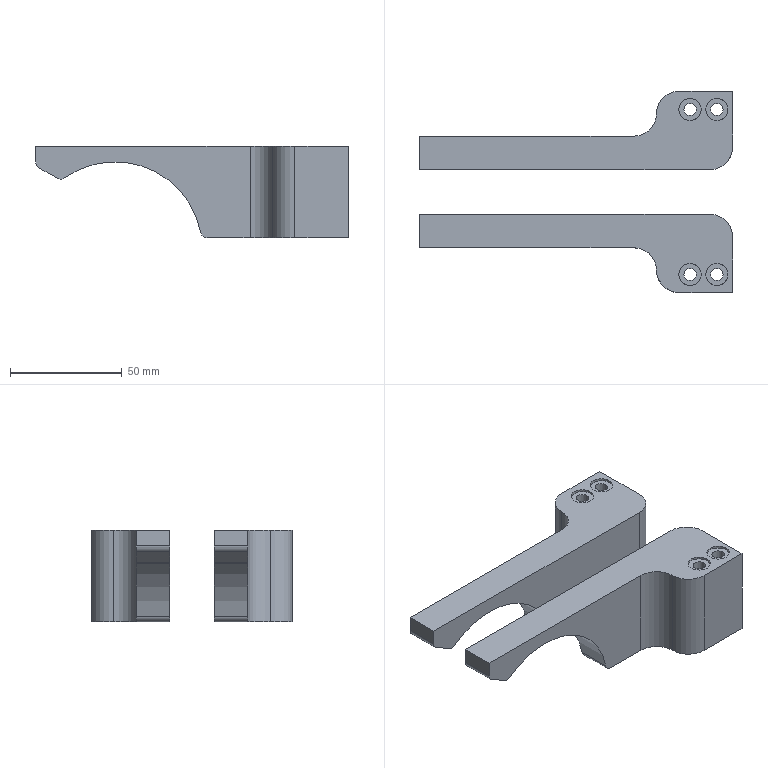NC program | NX | posted with a generic post | part box 140 x 90 x 41 mm
Lines 1 to 42 of 29499:
N10 G17 G21 G94 G90
(FLOOR_WALL_COPY , TOOL : D63)
N12 T01 M6
N14 G54
N16 G17 G0 G90 X109.5 Y0. S6500 M3
N18 G43 Z30. H1
N20 Z3.
N22 G94 G1 Z0. F1500.
N24 X106.5
N26 X-106.5
N28 X-109.5
N30 Z3.
N32 G0 Z30.
N34 M5
(DRILLING_COPY_1 , TOOL : D6A45)
N36 T07 M6
N38 G54
N40 G17 G0 G90 X51.003 Y-9.4 S5000 M3
N42 G43 Z30. H7
N44 G94 G81 G98 Z-1. F250. R3.
N46 X63.003
N48 G80
N50 G0 X63.003 Y-9.4 Z30.
N52 M5
(DRILLING_COPY_COPY , TOOL : 5.5ZT)
N54 T15 M6
N56 G54
N58 G17 G0 G90 X51.003 Y-9.4 S2000 M3
N60 G43 Z30. H15
N62 G94 G83 G98 Z-42.652 F200. Q2. R3.
N64 X63.003
N66 G80
N68 G0 X63.003 Y-9.4 Z30.
N70 M5